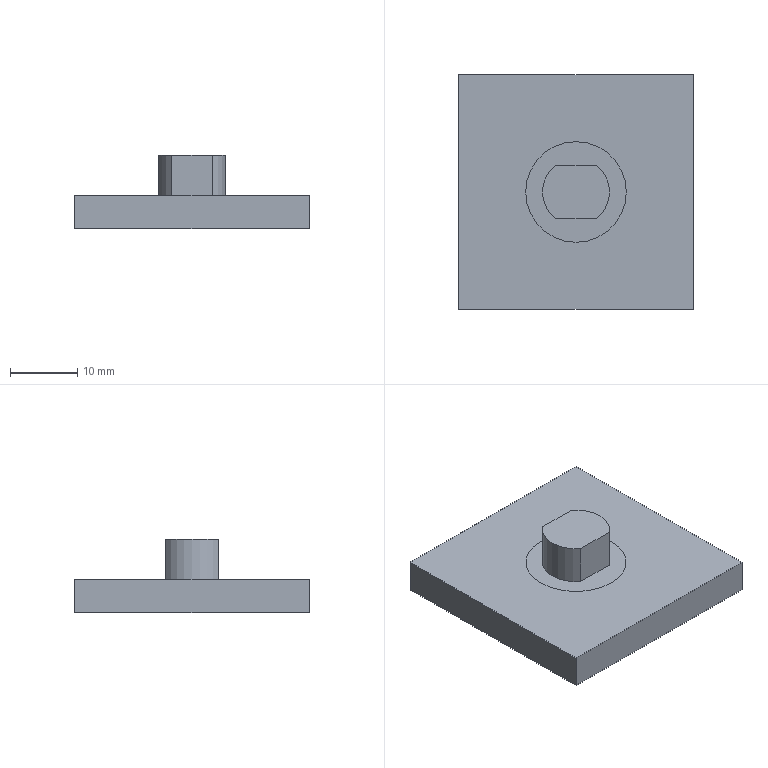NC program | NX | posted with a generic post | part box 35 x 35 x 11 mm
Whole program:
N10 G17 G21 G94 G90
(ZLEVEL_PROFILE , TOOL : D10)
N12 T10 M6
N14 G54
N16 G17 G0 G90 X6.132 Y-10.59 S3000 M3
N18 G43 Z30. H10
N20 Z-0.214
N22 G94 G1 X5.226 Y-9.413 F1000.
N24 G3 X4.302 Y-9.032 R1.
N26 G2 X3.041 Y-9.1 R8.049 F2000.
N28 G1 X-3.42
N30 G2 X-4.302 Y-9.032 R5.727
N32 G3 X-5.234 Y-9.392 R1.
N34 G1 X-6.182 Y-10.57
N36 G0 Z-0.429
N38 G1 X-5.234 Y-9.393 F1000.
N40 G2 X-4.302 Y-9.032 R1.
N42 G3 X-3.421 Y-9.1 R5.725 F2000.
N44 G1 X3.041
N46 G3 X4.302 Y-9.032 R8.046
N48 G2 X5.226 Y-9.413 R1.
N50 G1 X6.132 Y-10.59
N52 G0 Z-0.643
N54 G1 X5.226 Y-9.413 F1000.
N56 G3 X4.302 Y-9.032 R1.
N58 G2 X3.041 Y-9.1 R8.043 F2000.
N60 G1 X-3.423
N62 G2 X-4.302 Y-9.032 R5.723
N64 G3 X-5.234 Y-9.393 R1.
N66 G1 X-6.182 Y-10.57
N68 G0 X-6.181 Y-10.571 Z-0.857
N70 G1 X-5.234 Y-9.394 F1000.
N72 G2 X-4.302 Y-9.032 R1.
N74 G3 X-3.424 Y-9.1 R5.721 F2000.
N76 G1 X3.041
N78 G3 X4.302 Y-9.032 R8.042
N80 G2 X5.226 Y-9.414 R1.
N82 G1 X6.131 Y-10.591
N84 G0 Z-1.071
N86 G1 X5.226 Y-9.414 F1000.
N88 G3 X4.302 Y-9.032 R1.
N90 G2 X3.041 Y-9.1 R8.04 F2000.
N92 G1 X-3.426
N94 G2 X-4.302 Y-9.032 R5.719
N96 G3 X-5.234 Y-9.394 R1.
N98 G1 X-6.181 Y-10.571
N100 G0 X-6.18 Z-1.286
N102 G1 X-5.234 Y-9.394 F1000.
N104 G2 X-4.302 Y-9.033 R1.
N106 G3 X-3.427 Y-9.1 R5.717 F2000.
N108 G1 X3.041
N110 G3 X4.302 Y-9.033 R8.039
N112 G2 X5.226 Y-9.414 R1.
N114 G1 X6.131 Y-10.591
N116 G0 Z-1.5
N118 G1 X5.226 Y-9.415 F1000.
N120 G3 X4.302 Y-9.033 R1.
N122 G2 X3.041 Y-9.1 R8.037 F2000.
N124 G1 X-3.428
N126 G2 X-4.302 Y-9.033 R5.715
N128 G3 X-5.234 Y-9.395 R1.
N130 G1 X-6.18 Y-10.572
N132 G0 X-6.179 Z-1.714
N134 G1 X-5.234 Y-9.395 F1000.
N136 G2 X-4.302 Y-9.033 R1.
N138 G3 X-3.43 Y-9.1 R5.713 F2000.
N140 G1 X3.041
N142 G3 X4.302 Y-9.033 R8.036
N144 G2 X5.226 Y-9.415 R1.
N146 G1 X6.13 Y-10.592
N148 G0 Z-1.929
N150 G1 X5.226 Y-9.415 F1000.
N152 G3 X4.302 Y-9.033 R1.
N154 G2 X3.041 Y-9.1 R8.035 F2000.
N156 G1 X-3.438
N158 G2 X-4.302 Y-9.033 R5.623
N160 G3 X-5.234 Y-9.394 R1.
N162 G1 X-6.182 Y-10.571
N164 G0 Z-2.143
N166 G1 X-5.234 Y-9.394 F1000.
N168 G2 X-4.302 Y-9.033 R1.
N170 G3 X-3.441 Y-9.1 R5.601 F2000.
N172 G1 X3.041
N174 G3 X4.302 Y-9.033 R8.033
N176 G2 X5.226 Y-9.416 R1.
N178 G1 X6.13 Y-10.592
N180 G0 X6.129 Y-10.593 Z-2.357
N182 G1 X5.226 Y-9.416 F1000.
N184 G3 X4.302 Y-9.034 R1.
N186 G2 X3.041 Y-9.1 R8.032 F2000.
N188 G1 X-3.444
N190 G2 X-4.302 Y-9.034 R5.58
N192 G3 X-5.234 Y-9.395 R1.
N194 G1 X-6.182 Y-10.571
N196 G0 Y-10.572 Z-2.571
N198 G1 X-5.234 Y-9.395 F1000.
N200 G2 X-4.302 Y-9.034 R1.
N202 G3 X-3.447 Y-9.1 R5.559 F2000.
N204 G1 X3.041
N206 G3 X4.302 Y-9.034 R8.03
N208 G2 X5.226 Y-9.416 R1.
N210 G1 X6.129 Y-10.593
N212 G0 Z-2.786
N214 G1 X5.226 Y-9.417 F1000.
N216 G3 X4.302 Y-9.034 R1.
N218 G2 X3.041 Y-9.1 R8.029 F2000.
N220 G1 X-3.45
N222 G2 X-4.302 Y-9.034 R5.539
N224 G3 X-5.234 Y-9.395 R1.
N226 G1 X-6.182 Y-10.572
N228 G0 X-6.183 Z-3.
N230 G1 X-5.235 Y-9.395 F1000.
N232 G2 X-4.302 Y-9.034 R1.
N234 G3 X-3.452 Y-9.1 R5.518 F2000.
N236 G1 X3.041
N238 G3 X4.302 Y-9.034 R8.027
N240 G2 X5.226 Y-9.417 R1.
N242 G1 X6.128 Y-10.594
N244 G0 Z-3.214
N246 G1 X5.226 Y-9.417 F1000.
N248 G3 X4.302 Y-9.034 R1.
N250 G2 X3.041 Y-9.1 R8.026 F2000.
N252 G1 X-3.446
N254 G2 X-4.302 Y-9.034 R5.618
N256 G3 X-5.234 Y-9.397 R1.
N258 G1 X-6.179 Y-10.573
N260 G0 X-6.18 Z-3.429
N262 G1 X-5.234 Y-9.396 F1000.
N264 G2 X-4.302 Y-9.035 R1.
N266 G3 X-3.45 Y-9.1 R5.576 F2000.
N268 G1 X3.041
N270 G3 X4.302 Y-9.035 R8.025
N272 G2 X5.226 Y-9.418 R1.
N274 G1 X6.128 Y-10.594
N276 G0 Z-3.643
N278 G1 X5.226 Y-9.418 F1000.
N280 G3 X4.302 Y-9.035 R1.
N282 G2 X3.041 Y-9.1 R8.023 F2000.
N284 G1 X-3.455
N286 G2 X-4.302 Y-9.035 R5.533
N288 G3 X-5.234 Y-9.396 R1.
N290 G1 X-6.181 Y-10.573
N292 G0 X-6.182 Z-3.857
N294 G1 X-5.234 Y-9.396 F1000.
N296 G2 X-4.302 Y-9.035 R1.
N298 G3 X-3.46 Y-9.1 R5.489 F2000.
N300 G1 X3.041
N302 G3 X4.302 Y-9.035 R8.022
N304 G2 X5.226 Y-9.418 R1.
N306 G1 X6.127 Y-10.595
N308 G0 X6.19 Y-10.57 Z-4.071
N310 G1 X5.236 Y-9.393 F1000.
N312 G3 X4.302 Y-9.035 R1.
N314 G2 X3.481 Y-9.1 R5.232 F2000.
N316 G1 X-3.464
N318 G2 X-4.302 Y-9.035 R5.445
N320 G3 X-5.235 Y-9.396 R1.
N322 G1 X-6.182 Y-10.573
N324 G0 X-6.183 Y-10.572 Z-4.286
N326 G1 X-5.235 Y-9.396 F1000.
N328 G2 X-4.302 Y-9.035 R1.
N330 G3 X-3.469 Y-9.1 R5.4 F2000.
N332 G1 X3.484
N334 G3 X4.302 Y-9.035 R5.214
N336 G2 X5.236 Y-9.393 R1.
N338 G1 X6.19 Y-10.57
N340 G0 Z-4.5
N342 G1 X5.236 Y-9.393 F1000.
N344 G3 X4.302 Y-9.036 R1.
N346 G2 X3.486 Y-9.1 R5.197 F2000.
N348 G1 X-3.474
N350 G2 X-4.302 Y-9.036 R5.354
N352 G3 X-5.235 Y-9.396 R1.
N354 G1 X-6.184 Y-10.572
N356 G0 X-6.185 Z-4.714
N358 G1 X-5.235 Y-9.395 F1000.
N360 G2 X-4.302 Y-9.036 R1.
N362 G3 X-3.479 Y-9.1 R5.308 F2000.
N364 G1 X3.489
N366 G3 X4.302 Y-9.036 R5.18
N368 G2 X5.236 Y-9.394 R1.
N370 G1 X6.19 Y-10.57
N372 G0 Z-4.929
N374 G1 X5.236 Y-9.394 F1000.
N376 G3 X4.302 Y-9.036 R1.
N378 G2 X3.491 Y-9.1 R5.162 F2000.
N380 G1 X-3.484
N382 G2 X-4.302 Y-9.036 R5.261
N384 G3 X-5.235 Y-9.395 R1.
N386 G1 X-6.186 Y-10.572
N388 G0 X-6.188 Y-10.571 Z-5.143
N390 G1 X-5.236 Y-9.395 F1000.
N392 G2 X-4.302 Y-9.036 R1.
N394 G3 X-3.489 Y-9.1 R5.214 F2000.
N396 G1 X3.494
N398 G3 X4.302 Y-9.036 R5.145
N400 G2 X5.236 Y-9.394 R1.
N402 G1 X6.19 Y-10.57
N404 G0 Y-10.571 Z-5.357
N406 G1 X5.236 Y-9.394 F1000.
N408 G3 X4.302 Y-9.036 R1.
N410 G2 X3.497 Y-9.1 R5.128 F2000.
N412 G1 X-3.494
N414 G2 X-4.302 Y-9.036 R5.166
N416 G3 X-5.236 Y-9.395 R1.
N418 G1 X-6.189 Y-10.571
N420 G0 X-6.19 Z-5.571
N422 G1 X-5.236 Y-9.394 F1000.
N424 G2 X-4.302 Y-9.037 R1.
N426 G3 X-3.499 Y-9.1 R5.117 F2000.
N428 G1 X3.499
N430 G3 X4.302 Y-9.037 R5.11
N432 G2 X5.236 Y-9.394 R1.
N434 G1 X6.19 Y-10.571
N436 G0 X6.159 Y-10.583 Z-5.786
N438 G1 X5.211 Y-9.403 F1000.
N440 G3 X4.279 Y-9.04 R1.
N442 G2 X3.503 Y-9.1 R5.083 F2000.
N444 G1 X-3.504
N446 G2 X-4.302 Y-9.037 R5.068
N448 G3 X-5.236 Y-9.394 R1.
N450 G1 X-6.191 Y-10.571
N452 G0 X-6.153 Y-10.586 Z-6.
N454 G1 X-5.21 Y-9.405 F1000.
N456 G2 X-4.279 Y-9.041 R1.
N458 G3 X-3.492 Y-9.1 R5.245 F2000.
N460 G1 X3.505
N462 G3 X4.279 Y-9.041 R5.066
N464 G2 X5.211 Y-9.403 R1.
N466 G1 X6.159 Y-10.584
N468 G0 Z30.
N470 X-6.128 Y10.591
N472 Z-0.214
N474 G1 X-5.225 Y9.414 F1000.
N476 G3 X-4.302 Y9.032 R1.
N478 G2 X-3. Y9.1 R8.31 F2000.
N480 G1 X3.
N482 X3.887 Y9.022
N484 X3.945 Y9.076
N486 X4.302 Y9.032
N488 G3 X5.222 Y9.422 R1.
N490 G1 X6.11 Y10.599
N492 G0 Z-0.429
N494 G1 X5.222 Y9.422 F1000.
N496 G2 X4.302 Y9.032 R1.
N498 G1 X3.945 Y9.076 F2000.
N500 X3.887 Y9.022
N502 X3. Y9.1
N504 X-3.
N506 G3 X-4.302 Y9.032 R8.307
N508 G2 X-5.225 Y9.415 R1.
N510 G1 X-6.128 Y10.592
N512 G0 Z-0.643
N514 G1 X-5.225 Y9.415 F1000.
N516 G3 X-4.302 Y9.032 R1.
N518 G2 X-3. Y9.1 R8.305 F2000.
N520 G1 X3.
N522 X3.887 Y9.022
N524 X3.945 Y9.076
N526 X4.302 Y9.032
N528 G3 X5.222 Y9.422 R1.
N530 G1 X6.11 Y10.599
N532 G0 Z-0.857
N534 G1 X5.222 Y9.423 F1000.
N536 G2 X4.302 Y9.032 R1.
N538 G1 X3.945 Y9.076 F2000.
N540 X3.887 Y9.022
N542 X3. Y9.1
N544 X-3.
N546 G3 X-4.302 Y9.032 R8.303
N548 G2 X-5.225 Y9.415 R1.
N550 G1 X-6.128 Y10.592
N552 G0 X-6.127 Z-1.071
N554 G1 X-5.225 Y9.416 F1000.
N556 G3 X-4.302 Y9.032 R1.
N558 G2 X-3. Y9.1 R8.302 F2000.
N560 G1 X3.
N562 X3.887 Y9.022
N564 X3.945 Y9.076
N566 X4.302 Y9.032
N568 G3 X5.222 Y9.423 R1.
N570 G1 X6.11 Y10.599
N572 G0 Z-1.286
N574 G1 X5.222 Y9.423 F1000.
N576 G2 X4.302 Y9.033 R1.
N578 G1 X3.945 Y9.077 F2000.
N580 X3.887 Y9.022
N582 X3. Y9.1
N584 X-3.447
N586 G3 X-4.302 Y9.033 R5.459
N588 G2 X-5.235 Y9.391 R1.
N590 G1 X-6.189 Y10.568
N592 G0 Z-1.5
N594 G1 X-5.235 Y9.391 F1000.
N596 G3 X-4.302 Y9.033 R1.
N598 G2 X-3.45 Y9.1 R5.442 F2000.
N600 G1 X3.
N602 X3.887 Y9.022
N604 X3.945 Y9.077
N606 X4.302 Y9.033
N608 G3 X5.222 Y9.423 R1.
N610 G1 X6.11 Y10.6
N612 G0 Z-1.714
N614 G1 X5.222 Y9.423 F1000.
N616 G2 X4.302 Y9.033 R1.
N618 G1 X3.945 Y9.077 F2000.
N620 X3.887 Y9.022
N622 X3. Y9.1
N624 X-3.452
N626 G3 X-4.302 Y9.033 R5.424
N628 G2 X-5.235 Y9.391 R1.
N630 G1 X-6.189 Y10.568
N632 G0 Z-1.929
N634 G1 X-5.235 Y9.391 F1000.
N636 G3 X-4.302 Y9.033 R1.
N638 G2 X-3.455 Y9.1 R5.407 F2000.
N640 G1 X3.
N642 X3.887 Y9.022
N644 X3.945 Y9.077
N646 X4.302 Y9.033
N648 G3 X5.222 Y9.424 R1.
N650 G1 X6.11 Y10.6
N652 G0 Z-2.143
N654 G1 X5.222 Y9.424 F1000.
N656 G2 X4.302 Y9.033 R1.
N658 G1 X3.945 Y9.077 F2000.
N660 X3.887 Y9.022
N662 X3. Y9.1
N664 X-3.457
N666 G3 X-4.302 Y9.033 R5.389
N668 G2 X-5.235 Y9.392 R1.
N670 G1 X-6.189 Y10.568
N672 G0 Y10.569 Z-2.357
N674 G1 X-5.235 Y9.392 F1000.
N676 G3 X-4.302 Y9.034 R1.
N678 G2 X-3.46 Y9.1 R5.371 F2000.
N680 G1 X3.
N682 X3.887 Y9.022
N684 X3.945 Y9.078
N686 X4.302 Y9.034
N688 G3 X5.222 Y9.424 R1.
N690 G1 X6.11 Y10.6
N692 G0 Y10.601 Z-2.571
N694 G1 X5.222 Y9.424 F1000.
N696 G2 X4.302 Y9.034 R1.
N698 G1 X3.945 Y9.078 F2000.
N700 X3.887 Y9.022
N702 X3. Y9.1
N704 X-3.463
N706 G3 X-4.302 Y9.034 R5.354
N708 G2 X-5.236 Y9.392 R1.
N710 G1 X-6.189 Y10.569
N712 G0 Z-2.786
N714 G1 X-5.236 Y9.392 F1000.
N716 G3 X-4.302 Y9.034 R1.
N718 G2 X-3.465 Y9.1 R5.336 F2000.
N720 G1 X3.
N722 X3.887 Y9.022
N724 X3.945 Y9.078
N726 X4.302 Y9.034
N728 G3 X5.223 Y9.424 R1.
N730 G1 X6.11 Y10.601
N732 G0 Z-3.
N734 G1 X5.223 Y9.425 F1000.
N736 G2 X4.302 Y9.034 R1.
N738 G1 X3.945 Y9.078 F2000.
N740 X3.887 Y9.022
N742 X3. Y9.1
N744 X-3.468
N746 G3 X-4.302 Y9.034 R5.319
N748 G2 X-5.236 Y9.392 R1.
N750 G1 X-6.189 Y10.569
N752 G0 Z-3.214
N754 G1 X-5.236 Y9.392 F1000.
N756 G3 X-4.302 Y9.034 R1.
N758 G2 X-3.471 Y9.1 R5.301 F2000.
N760 G1 X3.
N762 X3.887 Y9.022
N764 X3.945 Y9.078
N766 X4.302 Y9.034
N768 G3 X5.223 Y9.425 R1.
N770 G1 X6.11 Y10.601
N772 G0 Z-3.429
N774 G1 X5.223 Y9.425 F1000.
N776 G2 X4.302 Y9.035 R1.
N778 G1 X3.945 Y9.079 F2000.
N780 X3.887 Y9.022
N782 X3. Y9.1
N784 X-3.473
N786 G3 X-4.302 Y9.035 R5.284
N788 G2 X-5.236 Y9.393 R1.
N790 G1 X-6.189 Y10.569
N792 G0 Z-3.643
N794 G1 X-5.236 Y9.393 F1000.
N796 G3 X-4.302 Y9.035 R1.
N798 G2 X-3.476 Y9.1 R5.267 F2000.
N800 G1 X3.
N802 X3.887 Y9.022
N804 X3.945 Y9.079
N806 X4.302 Y9.035
N808 G3 X5.223 Y9.425 R1.
N810 G1 X6.11 Y10.602
N812 G0 Z-3.857
N814 G1 X5.223 Y9.425 F1000.
N816 G2 X4.302 Y9.035 R1.
N818 G1 X3.945 Y9.079 F2000.
N820 X3.887 Y9.022
N822 X3. Y9.1
N824 X-3.478
N826 G3 X-4.302 Y9.035 R5.249
N828 G2 X-5.236 Y9.393 R1.
N830 G1 X-6.19 Y10.57
N832 G0 Z-4.071
N834 G1 X-5.236 Y9.393 F1000.
N836 G3 X-4.302 Y9.035 R1.
N838 G2 X-3.481 Y9.1 R5.232 F2000.
N840 G1 X3.
N842 X3.887 Y9.022
N844 X3.945 Y9.079
N846 X4.302 Y9.035
N848 G3 X5.223 Y9.426 R1.
N850 G1 X6.11 Y10.602
N852 G0 Z-4.286
N854 G1 X5.223 Y9.426 F1000.
N856 G2 X4.302 Y9.035 R1.
N858 G1 X3.945 Y9.079 F2000.
N860 X3.887 Y9.022
N862 X3. Y9.1
N864 X-3.484
N866 G3 X-4.302 Y9.035 R5.214
N868 G2 X-5.236 Y9.393 R1.
N870 G1 X-6.19 Y10.57
N872 G0 Z-4.5
N874 G1 X-5.236 Y9.393 F1000.
N876 G3 X-4.302 Y9.036 R1.
N878 G2 X-3.486 Y9.1 R5.197 F2000.
N880 G1 X3.
N882 X3.887 Y9.022
N884 X3.945 Y9.079
N886 X4.302 Y9.036
N888 G3 X5.223 Y9.426 R1.
N890 G1 X6.11 Y10.602
N892 G0 Z-4.714
N894 G1 X5.223 Y9.426 F1000.
N896 G2 X4.302 Y9.036 R1.
N898 G1 X3.945 Y9.08 F2000.
N900 X3.887 Y9.022
N902 X3. Y9.1
N904 X-3.489
N906 G3 X-4.302 Y9.036 R5.18
N908 G2 X-5.236 Y9.394 R1.
N910 G1 X-6.19 Y10.57
N912 G0 Z-4.929
N914 G1 X-5.236 Y9.394 F1000.
N916 G3 X-4.302 Y9.036 R1.
N918 G2 X-3.491 Y9.1 R5.162 F2000.
N920 G1 X3.
N922 X3.887 Y9.022
N924 X3.945 Y9.08
N926 X4.302 Y9.036
N928 G3 X5.223 Y9.426 R1.
N930 G1 X6.11 Y10.603
N932 G0 Z-5.143
N934 G1 X5.223 Y9.427 F1000.
N936 G2 X4.302 Y9.036 R1.
N938 G1 X3.945 Y9.08 F2000.
N940 X3.887 Y9.022
N942 X3. Y9.1
N944 X-3.494
N946 G3 X-4.302 Y9.036 R5.145
N948 G2 X-5.236 Y9.394 R1.
N950 G1 X-6.19 Y10.57
N952 G0 Y10.571 Z-5.357
N954 G1 X-5.236 Y9.394 F1000.
N956 G3 X-4.302 Y9.036 R1.
N958 G2 X-3.497 Y9.1 R5.128 F2000.
N960 G1 X3.
N962 X3.887 Y9.022
N964 X3.946 Y9.08
N966 X4.302 Y9.036
N968 G3 X5.223 Y9.427 R1.
N970 G1 X6.11 Y10.603
N972 G0 X6.109 Z-5.571
N974 G1 X5.223 Y9.427 F1000.
N976 G2 X4.302 Y9.037 R1.
N978 G1 X3.946 Y9.08 F2000.
N980 X3.887 Y9.022
N982 X3. Y9.1
N984 X-3.499
N986 G3 X-4.302 Y9.037 R5.11
N988 G2 X-5.236 Y9.394 R1.
N990 G1 X-6.19 Y10.571
N992 G0 Z-5.786
N994 G1 X-5.236 Y9.394 F1000.
N996 G3 X-4.302 Y9.037 R1.
N998 G2 X-3.502 Y9.1 R5.093 F2000.
N1000 G1 X3.
N1002 X3.84 Y9.03
N1004 X3.846 Y9.088
N1006 X3.897 Y9.113
N1008 X3.946 Y9.081
N1010 X4.302 Y9.037
N1012 G3 X5.223 Y9.427 R1.
N1014 G1 X6.109 Y10.603
N1016 G0 X6.083 Y10.614 Z-6.
N1018 G1 X5.198 Y9.434 F1000.
N1020 G2 X4.279 Y9.041 R1.
N1022 G1 X3.946 Y9.081 F2000.
N1024 X3.898 Y9.115
N1026 X3.844 Y9.089
N1028 X3.84 Y9.03
N1030 X3. Y9.1
N1032 X-3.505
N1034 G3 X-4.279 Y9.041 R5.066
N1036 G2 X-5.211 Y9.403 R1.
N1038 G1 X-6.159 Y10.584
N1040 G0 Z30.
N1042 M5
(ZLEVEL_PROFILE_COPY , TOOL : D10JING)
N1044 T11 M6
N1046 G54
N1048 G17 G0 G90 X5.985 Y-10.544 S5000 M3
N1050 G43 Z30. H11
N1052 Z-6.
N1054 G94 G1 X5.067 Y-9.343 F1000.
N1056 G3 X4.144 Y-8.958 R1.
N1058 G2 X3.5 Y-9. R5.004
N1060 G1 X-3.515
N1062 G2 X-4.144 Y-8.958 R4.77
N1064 G3 X-5.068 Y-9.34 R1.
N1066 G1 X-5.993 Y-10.541
N1068 G0 Z30.
N1070 X-5.985 Y10.544
N1072 Z-6.
N1074 G1 X-5.067 Y9.343
N1076 G3 X-4.144 Y8.958 R1.
N1078 G2 X-3.5 Y9. R5.004
N1080 G1 X3.515
N1082 G2 X4.144 Y8.958 R4.77
N1084 G3 X5.068 Y9.34 R1.
N1086 G1 X5.993 Y10.541
N1088 G0 Z30.
N1090 M5
(PLANAR_MILL_COPY , TOOL : D6A45)
N1092 T07 M6
N1094 G54
N1096 G17 G0 G90 X3.866 Y-5.4 S7500 M3
N1098 G43 Z30. H7
N1100 Z0.5
N1102 G94 G1 Z-1. F1400.
N1104 G3 X3. Y-4.9 R1.
N1106 G1 X-3.
N1108 G3 X-3.866 Y-5.4 R1.
N1110 G1 Z0.5
N1112 G0 Z30.
N1114 Y5.4
N1116 Z0.5
N1118 G1 Z-1.
N1120 G3 X-3. Y4.9 R1.
N1122 G1 X3.
N1124 G3 X3.866 Y5.4 R1.
N1126 G1 Z0.5
N1128 G0 Z30.
N1130 M5
N1132 M2